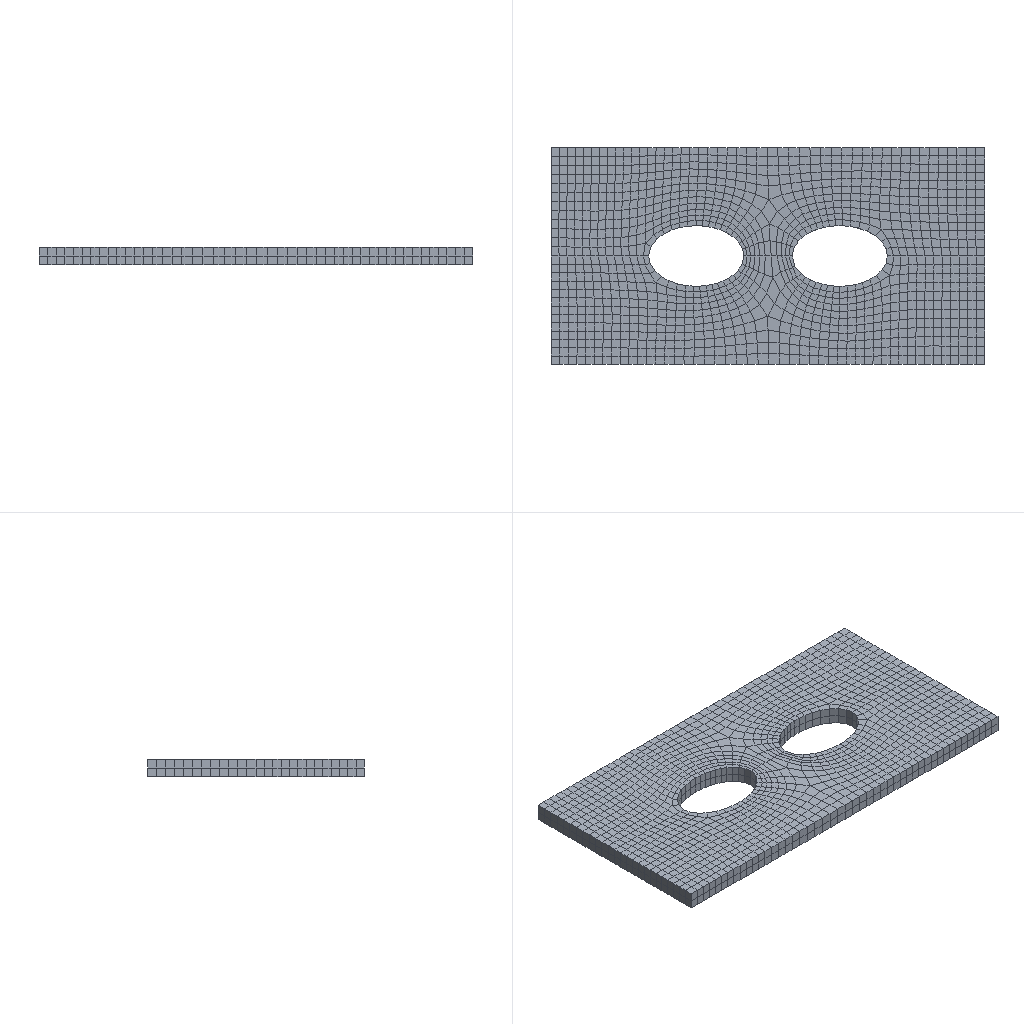Simulation study | abaqus
Set-up summary:
category,name,step,type,value,unit,region
solver,abaqus
solver,version,,,Abaqus/Standard 2020
units,not stated in the deck,,not stated
analysis,deck,,coupled temperature-displacement,coupled temperature-displacement
load_step,Step-1,Step-1,coupled temperature-displacement
load_step,requested,,,1
mesh,nodes,,,3882
mesh,elements,,,2378
element_type,Q3D8,,solid,2378
load,load commands in deck,,count,4
bc,support commands in deck,,count,4
material,MATERIAL-1,,in results
check,setup vs results,,match,"per instance, exact: element labels, types and connectivity; labels of the nodes the elements use; coordinates of those nodes at SINGLE_PRECISION in 1 of 1 instance(s)"
Abaqus input file, long lists of numbers shortened:
*Heading
** Job name: Job-2 Model name: Model-1-Copy
** Generated by: Abaqus/CAE 2020
*Preprint, echo=NO, model=NO, history=NO, contact=NO
**
** PARTS
**
*Part, name=work
*Node
      1,           0.,         -25.,           0.
      2,           0.,        -12.5,           0.
** (3880 more lines like these left out)
*Element, type=Q3D8
   1,  537,  538,  116,  115, 2870, 2871, 1643, 1644
   2,  538,  502,  117,  116, 2871, 2835, 1642, 1643
** (2376 more lines like these left out)
*Nset, nset=Set-3, generate
    1,  3882,     1
*Elset, elset=Set-3, generate
    1,  2378,     1
*Nset, nset=Set-fix
  134,  194, 1651
*Nset, nset=fixfix
  131,  132,  133,  134,  135,  136,  192,  193,  194,  195,  196,  197, 1649, 1650, 1651, 1652
 1653, 1654
*Nset, nset=Set-ff
  131,  136,  192,  197,  771,  776,  777,  781, 1288, 1293, 1294, 1298, 1649, 1654, 1928, 1932
 1937, 1938, 1941, 1945, 2460, 2464, 2469, 2470, 2473, 2477, 3104, 3109, 3110, 3114, 3610, 3614
** (1 more lines like these left out)
** Section: Section-1
*Solid Section, elset=Set-3, material=Material-1
,
*End Part
**
**
** ASSEMBLY
**
*Assembly, name=Assembly
**
*Instance, name=work-1, part=work
*End Instance
**
*Nset, nset=Set-1, instance=work-1
    1,    4,    5,    8,   15,   16,   17,   18,   19,   20,   43,   44,   45,   46,   47,   48
   49,   50,   51,   52,   53,   54,   55,   56,   57,   58,   59,   60,   61,   62,   63,   64
** (17 more lines like these left out)
*Elset, elset=Set-1, instance=work-1
   12,   22,   23,   24,   25,   26,   27,   28,   29,   30,   31,   32,   33,   34,  192,  203
  214,  225,  236,  247,  258,  269,  280,  381,  382,  383,  384,  385,  386,  387,  388,  389
** (10 more lines like these left out)
*Nset, nset=Set-6, instance=work-1
    1,    8,   15,   16,   43,   44,   45,   46,   47,   48,   49,   50,   51,   52,   53,   54
   55,   56,   57,   58,   59,   60,   61,   62,   63,   64,   65,   66,   67,   68,   69,   70
** (7 more lines like these left out)
*Elset, elset=Set-6, instance=work-1
   12,   22,   23,   24,   25,   26,   27,   28,   29,   30,   31,   32,   33,   34,  192,  203
  214,  225,  236,  247,  258,  269,  280,  381,  382,  383,  384,  385,  386,  387,  388,  389
** (4 more lines like these left out)
*Nset, nset=Set-11, instance=work-1
    4,    5,   11,   12,  129,  130,  131,  132,  133,  134,  135,  136,  137,  138,  159,  162
  190,  191,  192,  193,  194,  195,  196,  197,  198,  199, 1647, 1648, 1649, 1650, 1651, 1652
** (1 more lines like these left out)
*Elset, elset=Set-11, instance=work-1
  295,  296,  297,  298,  299,  300,  301,  302,  303,  304,  305,  882,  883,  884,  885,  886
  887,  888,  889,  890,  891,  892, 1449, 1451, 1453, 1455, 1457, 1458, 1459, 1460, 1461, 1462
** (1 more lines like these left out)
*Elset, elset=_Surf-1_S4, internal, instance=work-1
   12,   22,  192,  203,  214,  225,  236,  247,  258,  269,  280,  487,  497,  507,  517,  527
  537,  547,  557,  567,  577,  587,  599,  609,  779,  790,  801,  812,  823,  834,  845,  856
** (4 more lines like these left out)
*Elset, elset=_Surf-1_S5, internal, instance=work-1
   23,   24,   25,   26,   27,   28,   29,   30,   31,   32,   33,   34,  388,  389,  390,  391
  392,  393,  610,  611,  612,  613,  614,  615,  616,  617,  618,  619,  620,  621,  975,  976
** (3 more lines like these left out)
*Elset, elset=_Surf-1_S3, internal, instance=work-1
  381,  382,  383,  384,  385,  386,  387,  968,  969,  970,  971,  972,  973,  974, 1553, 1554
 1555, 1556, 1557, 1558, 1559, 2155, 2156, 2157, 2158, 2159, 2160, 2161
*Surface, type=ELEMENT, name=Surf-1
_Surf-1_S4, S4
_Surf-1_S5, S5
_Surf-1_S3, S3
*Elset, elset=_Surf-2_S4, internal, instance=work-1
   12,   22,  192,  203,  214,  225,  236,  247,  258,  269,  280,  487,  497,  507,  517,  527
  537,  547,  557,  567,  577,  587,  599,  609,  779,  790,  801,  812,  823,  834,  845,  856
** (4 more lines like these left out)
*Elset, elset=_Surf-2_S5, internal, instance=work-1
   23,   24,   25,   26,   27,   28,   29,   30,   31,   32,   33,   34,  388,  389,  390,  391
  392,  393,  610,  611,  612,  613,  614,  615,  616,  617,  618,  619,  620,  621,  975,  976
** (3 more lines like these left out)
*Elset, elset=_Surf-2_S3, internal, instance=work-1
  381,  382,  383,  384,  385,  386,  387,  968,  969,  970,  971,  972,  973,  974, 1553, 1554
 1555, 1556, 1557, 1558, 1559, 2155, 2156, 2157, 2158, 2159, 2160, 2161
*Surface, type=ELEMENT, name=Surf-2
_Surf-2_S4, S4
_Surf-2_S5, S5
_Surf-2_S3, S3
*Elset, elset=_Surf-3_S4, internal, instance=work-1
   12,   22,  192,  203,  214,  225,  236,  247,  258,  269,  280,  487,  497,  507,  517,  527
  537,  547,  557,  567,  577,  587,  599,  609,  779,  790,  801,  812,  823,  834,  845,  856
** (4 more lines like these left out)
*Elset, elset=_Surf-3_S5, internal, instance=work-1
   23,   24,   25,   26,   27,   28,   29,   30,   31,   32,   33,   34,  388,  389,  390,  391
  392,  393,  610,  611,  612,  613,  614,  615,  616,  617,  618,  619,  620,  621,  975,  976
** (3 more lines like these left out)
*Elset, elset=_Surf-3_S3, internal, instance=work-1
  381,  382,  383,  384,  385,  386,  387,  968,  969,  970,  971,  972,  973,  974, 1553, 1554
 1555, 1556, 1557, 1558, 1559, 2155, 2156, 2157, 2158, 2159, 2160, 2161
*Surface, type=ELEMENT, name=Surf-3
_Surf-3_S4, S4
_Surf-3_S5, S5
_Surf-3_S3, S3
*Elset, elset=_Surf-4_S4, internal, instance=work-1
   12,   22,  192,  203,  214,  225,  236,  247,  258,  269,  280,  487,  497,  507,  517,  527
  537,  547,  557,  567,  577,  587,  599,  609,  779,  790,  801,  812,  823,  834,  845,  856
** (4 more lines like these left out)
*Elset, elset=_Surf-4_S5, internal, instance=work-1
   23,   24,   25,   26,   27,   28,   29,   30,   31,   32,   33,   34,  388,  389,  390,  391
  392,  393,  610,  611,  612,  613,  614,  615,  616,  617,  618,  619,  620,  621,  975,  976
** (3 more lines like these left out)
*Elset, elset=_Surf-4_S3, internal, instance=work-1
  381,  382,  383,  384,  385,  386,  387,  968,  969,  970,  971,  972,  973,  974, 1553, 1554
 1555, 1556, 1557, 1558, 1559, 2155, 2156, 2157, 2158, 2159, 2160, 2161
*Surface, type=ELEMENT, name=Surf-4
_Surf-4_S4, S4
_Surf-4_S5, S5
_Surf-4_S3, S3
*Elset, elset=_Surf-5_S4, internal, instance=work-1
 1186, 1196, 1353, 1364, 1375, 1386, 1397, 1408, 1419, 1430, 1441, 1655, 1666, 1677, 1688, 1699
 1710, 1721, 1732, 1743, 1754, 1765, 1776, 1788, 1798, 1955, 1966, 1977, 1988, 1999, 2010, 2021
** (1 more lines like these left out)
*Elset, elset=_Surf-5_S5, internal, instance=work-1
 1197, 1198, 1199, 1200, 1201, 1202, 1203, 1204, 1205, 1206, 1207, 1560, 1561, 1562, 1563, 1564
 1565, 1799, 1800, 1801, 1802, 1803, 1804, 1805, 1806, 1807, 1808, 1809, 2162, 2163, 2164, 2165
** (1 more lines like these left out)
*Elset, elset=_Surf-5_S3, internal, instance=work-1
 1553, 1554, 1555, 1556, 1557, 1558, 1559, 2155, 2156, 2157, 2158, 2159, 2160, 2161
*Surface, type=ELEMENT, name=Surf-5
_Surf-5_S4, S4
_Surf-5_S5, S5
_Surf-5_S3, S3
*Elset, elset=_Surf-6_S4, internal, instance=work-1
   12,   22,  192,  203,  214,  225,  236,  247,  258,  269,  280,  487,  497,  507,  517,  527
  537,  547,  557,  567,  577,  587,  599,  609,  779,  790,  801,  812,  823,  834,  845,  856
** (4 more lines like these left out)
*Elset, elset=_Surf-6_S5, internal, instance=work-1
   23,   24,   25,   26,   27,   28,   29,   30,   31,   32,   33,   34,  388,  389,  390,  391
  392,  393,  610,  611,  612,  613,  614,  615,  616,  617,  618,  619,  620,  621,  975,  976
** (3 more lines like these left out)
*Elset, elset=_Surf-6_S3, internal, instance=work-1
  381,  382,  383,  384,  385,  386,  387,  968,  969,  970,  971,  972,  973,  974, 1553, 1554
 1555, 1556, 1557, 1558, 1559, 2155, 2156, 2157, 2158, 2159, 2160, 2161
*Surface, type=ELEMENT, name=Surf-6
_Surf-6_S4, S4
_Surf-6_S5, S5
_Surf-6_S3, S3
*End Assembly
*Amplitude, name=Amp-1, definition=PERIODIC
1,         188000.,              0.,              0.
             1.,              0.
*Amplitude, name=Amp-2
             0.,              0.,             10.,              1.
**
** MATERIALS
**
*Material, name=Material-1
*Conductivity
40.,
*Density
 1.67e-09,
*Elastic
70000., 0.33
*Electrical Conductivity
 0.02665,
*Expansion
 2.32e-06,
*Specific Heat
 8.9e+08,
**
** PHYSICAL CONSTANTS
**
*Physical Constants, absolute zero=-273., stefan boltzmann=5.67e-08
**
** BOUNDARY CONDITIONS
**
** Name: BC-4 Type: 对称/反对称/完全固定
*Boundary
work-1.Set-ff, ENCASTRE
**
** PREDEFINED FIELDS
**
** Name: Predefined Field-1   Type: Temperature
*Initial Conditions, type=TEMPERATURE
Set-1, 20.
** ----------------------------------------------------------------
**
** STEP: Step-1
**
*Step, name=Step-1, nlgeom=YES, inc=1000
*Coupled Temperature-displacement, electrical, creep=none, deltmx=1e+20, stabilize=0.0002, allsdtol=0.05, continue=NO
0.1, 10., 0.0001, 10.
**
** BOUNDARY CONDITIONS
**
** Name: BC-3 Type: 电势
*Boundary
work-1.fixfix, 9, 9
**
** LOADS
**
** Name: Load-1   Type: Surface current
*Dsecurrent, amplitude=Amp-1
Surf-6,CS,1.
** Name: Load-2   Type: Pressure
*Dsload, amplitude=Amp-2
Surf-4, P, 0.1
**
** INTERACTIONS
**
** Interaction: Int-1
*Sfilm
Surf-1, F, 20., 0.01
** Interaction: Int-2
*Sradiate
Surf-2, R, 20., 0.5
**
** OUTPUT REQUESTS
**
*Restart, write, frequency=0
**
** FIELD OUTPUT: F-Output-1
**
*Output, field
*Node Output
CECHG, CECUR, EPOT, NT, RECUR, RF, RFL, RT
U
*Element Output, directions=YES
E, ECD, EPG, HFL, LE, MISES, MISESMAX, NCURS, PE, PEEQ, S, TEMP, VE, VEEQ
*Contact Output
ECD, ECDA, ECDT, ECDTA
**
** HISTORY OUTPUT: H-Output-1
**
*Output, history, variable=PRESELECT
*End Step
Results summary:
result,step,,completed,increments=12 time=10.0/10.0
result,analysis,,,"coupled temperature-displacement, steady state"
result,last_loadstep,,,1
result,primary field,,,"U, NT11"
result,reaction total,,FX,-4e-06,model units
result,reaction total,,FY,0.0,model units
result,reaction total,,FZ,1e-06,model units